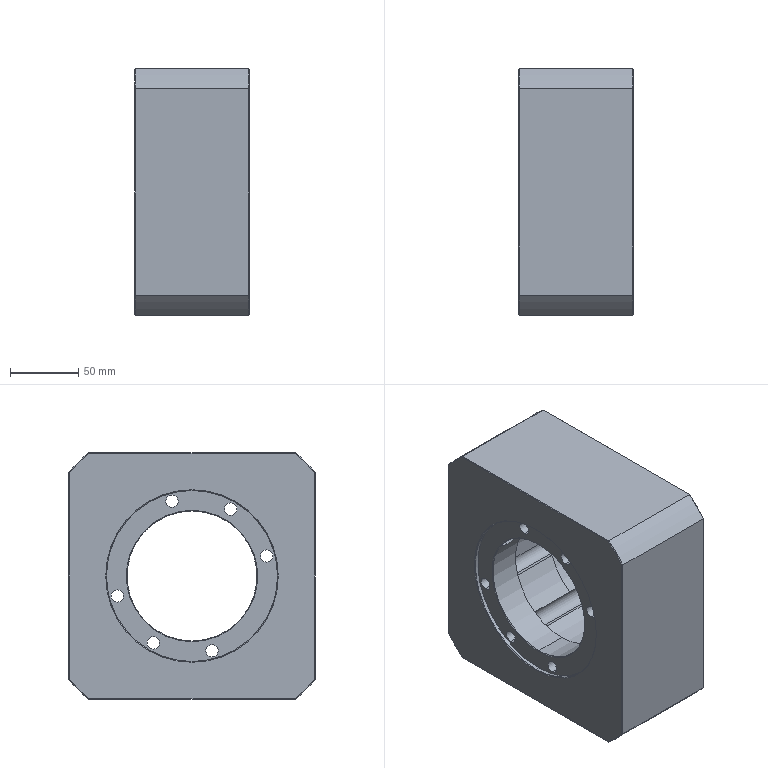Part | SolidWorks | features BaseBody 1 | 1 solid | 110 faces | box 84 x 180 x 180 mm | volume 1847787 mm3 | cylinder 56 | plane 28 | cone 26 | commonest cylinder face diameters 9 x12 14 x12 10.2 x8 112 x7 114.3 x7 235 x4